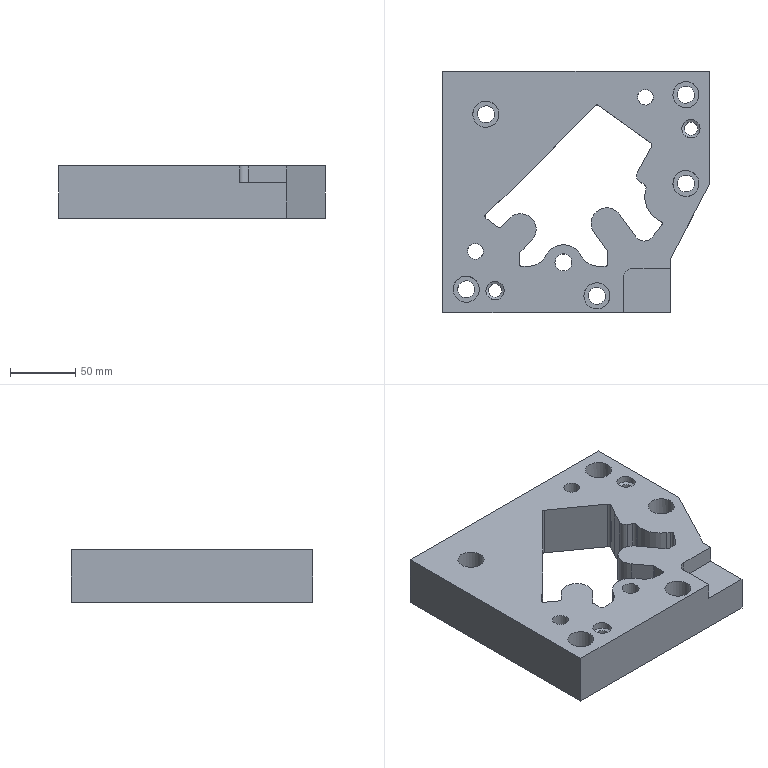Part | STEP file | gslz 2016.10.28-13_id118_x_t | 1 solid | 77 faces | box 204 x 185 x 40 mm | volume 1012043 mm3 | cylinder 38 | plane 37 | cone 2 | commonest cylinder face diameters 4 x9 13 x6 20 x5 30 x4 14 x3 10.3 x2